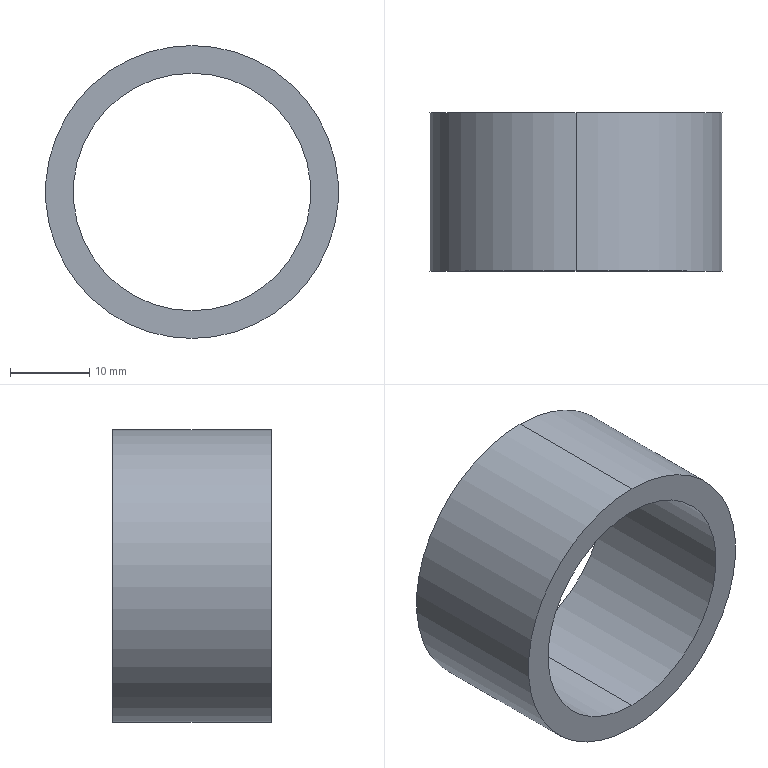Part | SolidWorks | features BaseBody 1 | 1 solid | 6 faces | box 37 x 20 x 37 mm | volume 7367 mm3 | cylinder 4 | plane 2 | commonest cylinder face diameters 30 x2 37 x2
STEP:
#1=CARTESIAN_POINT('',(-1069.592,-42.18,74.5));
#2=VERTEX_POINT('',#1);
#3=CARTESIAN_POINT('',(-1069.592,-22.18,74.5));
#4=VERTEX_POINT('',#3);
#5=CARTESIAN_POINT('',(-1069.592,-42.18,74.5));
#6=DIRECTION('',(0.,1.,0.));
#7=VECTOR('',#6,1000.);
#8=LINE('',#5,#7);
#9=EDGE_CURVE('',#2,#4,#8,.T.);
#10=ORIENTED_EDGE('',*,*,#9,.F.);
#11=CARTESIAN_POINT('',(-1069.592,-42.18,104.5));
#12=VERTEX_POINT('',#11);
#13=CARTESIAN_POINT('',(-1069.592,-42.18,89.5));
#14=DIRECTION('',(0.,1.,0.));
#15=DIRECTION('',(0.,0.,1.));
#16=AXIS2_PLACEMENT_3D('',#13,#14,#15);
#17=CIRCLE('',#16,15.);
#18=EDGE_CURVE('',#12,#2,#17,.T.);
#19=ORIENTED_EDGE('',*,*,#18,.F.);
#20=CARTESIAN_POINT('',(-1069.592,-22.18,104.5));
#21=VERTEX_POINT('',#20);
#22=CARTESIAN_POINT('',(-1069.592,-42.18,104.5));
#23=DIRECTION('',(0.,1.,0.));
#24=VECTOR('',#23,1000.);
#25=LINE('',#22,#24);
#26=EDGE_CURVE('',#12,#21,#25,.T.);
#27=ORIENTED_EDGE('',*,*,#26,.T.);
#28=CARTESIAN_POINT('',(-1069.592,-22.18,89.5));
#29=DIRECTION('',(0.,1.,0.));
#30=DIRECTION('',(0.,0.,1.));
#31=AXIS2_PLACEMENT_3D('',#28,#29,#30);
#32=CIRCLE('',#31,15.);
#33=EDGE_CURVE('',#21,#4,#32,.T.);
#34=ORIENTED_EDGE('',*,*,#33,.T.);
#35=EDGE_LOOP('',(#10,#19,#27,#34));
#36=FACE_OUTER_BOUND('',#35,.T.);
#37=CARTESIAN_POINT('',(-1069.592,-42.18,89.5));
#38=DIRECTION('',(0.,1.,0.));
#39=DIRECTION('',(0.,0.,1.));
#40=AXIS2_PLACEMENT_3D('',#37,#38,#39);
#41=CYLINDRICAL_SURFACE('',#40,15.);
#42=ADVANCED_FACE('',(#36),#41,.F.);
#43=CARTESIAN_POINT('',(-1069.592,-42.18,108.));
#44=VERTEX_POINT('',#43);
#45=CARTESIAN_POINT('',(-1069.592,-42.18,71.));
#46=VERTEX_POINT('',#45);
#47=CARTESIAN_POINT('',(-1069.592,-42.18,89.5));
#48=DIRECTION('',(0.,1.,0.));
#49=DIRECTION('',(0.,0.,1.));
#50=AXIS2_PLACEMENT_3D('',#47,#48,#49);
#51=CIRCLE('',#50,18.5);
#52=EDGE_CURVE('',#44,#46,#51,.T.);
#53=ORIENTED_EDGE('',*,*,#52,.F.);
#54=CARTESIAN_POINT('',(-1069.592,-42.18,89.5));
#55=DIRECTION('',(0.,1.,0.));
#56=DIRECTION('',(0.,0.,1.));
#57=AXIS2_PLACEMENT_3D('',#54,#55,#56);
#58=CIRCLE('',#57,18.5);
#59=EDGE_CURVE('',#46,#44,#58,.T.);
#60=ORIENTED_EDGE('',*,*,#59,.F.);
#61=EDGE_LOOP('',(#53,#60));
#62=FACE_OUTER_BOUND('',#61,.T.);
#63=ORIENTED_EDGE('',*,*,#18,.T.);
#64=CARTESIAN_POINT('',(-1069.592,-42.18,89.5));
#65=DIRECTION('',(0.,1.,0.));
#66=DIRECTION('',(0.,0.,1.));
#67=AXIS2_PLACEMENT_3D('',#64,#65,#66);
#68=CIRCLE('',#67,15.);
#69=EDGE_CURVE('',#2,#12,#68,.T.);
#70=ORIENTED_EDGE('',*,*,#69,.T.);
#71=EDGE_LOOP('',(#63,#70));
#72=FACE_BOUND('',#71,.T.);
#73=CARTESIAN_POINT('',(-1069.592,-42.18,89.5));
#74=DIRECTION('',(0.,-1.,0.));
#75=DIRECTION('',(-1.,0.,0.));
#76=AXIS2_PLACEMENT_3D('',#73,#74,#75);
#77=PLANE('',#76);
#78=ADVANCED_FACE('',(#62,#72),#77,.T.);
#79=CARTESIAN_POINT('',(-1069.592,-22.18,108.));
#80=VERTEX_POINT('',#79);
#81=CARTESIAN_POINT('',(-1069.592,-22.18,71.));
#82=VERTEX_POINT('',#81);
#83=CARTESIAN_POINT('',(-1069.592,-22.18,89.5));
#84=DIRECTION('',(0.,-1.,0.));
#85=DIRECTION('',(0.,0.,1.));
#86=AXIS2_PLACEMENT_3D('',#83,#84,#85);
#87=CIRCLE('',#86,18.5);
#88=EDGE_CURVE('',#80,#82,#87,.T.);
#89=ORIENTED_EDGE('',*,*,#88,.F.);
#90=CARTESIAN_POINT('',(-1069.592,-22.18,89.5));
#91=DIRECTION('',(0.,-1.,0.));
#92=DIRECTION('',(0.,0.,1.));
#93=AXIS2_PLACEMENT_3D('',#90,#91,#92);
#94=CIRCLE('',#93,18.5);
#95=EDGE_CURVE('',#82,#80,#94,.T.);
#96=ORIENTED_EDGE('',*,*,#95,.F.);
#97=EDGE_LOOP('',(#89,#96));
#98=FACE_OUTER_BOUND('',#97,.T.);
#99=ORIENTED_EDGE('',*,*,#33,.F.);
#100=CARTESIAN_POINT('',(-1069.592,-22.18,89.5));
#101=DIRECTION('',(0.,1.,0.));
#102=DIRECTION('',(0.,0.,1.));
#103=AXIS2_PLACEMENT_3D('',#100,#101,#102);
#104=CIRCLE('',#103,15.);
#105=EDGE_CURVE('',#4,#21,#104,.T.);
#106=ORIENTED_EDGE('',*,*,#105,.F.);
#107=EDGE_LOOP('',(#99,#106));
#108=FACE_BOUND('',#107,.T.);
#109=CARTESIAN_POINT('',(-1069.592,-22.18,89.5));
#110=DIRECTION('',(0.,-1.,0.));
#111=DIRECTION('',(-1.,0.,0.));
#112=AXIS2_PLACEMENT_3D('',#109,#110,#111);
#113=PLANE('',#112);
#114=ADVANCED_FACE('',(#98,#108),#113,.F.);
#115=CARTESIAN_POINT('',(-1069.592,-42.18,71.));
#116=DIRECTION('',(0.,1.,0.));
#117=VECTOR('',#116,1000.);
#118=LINE('',#115,#117);
#119=EDGE_CURVE('',#46,#82,#118,.T.);
#120=ORIENTED_EDGE('',*,*,#119,.F.);
#121=ORIENTED_EDGE('',*,*,#59,.T.);
#122=CARTESIAN_POINT('',(-1069.592,-42.18,108.));
#123=DIRECTION('',(0.,1.,0.));
#124=VECTOR('',#123,1000.);
#125=LINE('',#122,#124);
#126=EDGE_CURVE('',#44,#80,#125,.T.);
#127=ORIENTED_EDGE('',*,*,#126,.T.);
#128=ORIENTED_EDGE('',*,*,#88,.T.);
#129=EDGE_LOOP('',(#120,#121,#127,#128));
#130=FACE_OUTER_BOUND('',#129,.T.);
#131=CARTESIAN_POINT('',(-1069.592,-42.18,89.5));
#132=DIRECTION('',(0.,1.,0.));
#133=DIRECTION('',(0.,0.,1.));
#134=AXIS2_PLACEMENT_3D('',#131,#132,#133);
#135=CYLINDRICAL_SURFACE('',#134,18.5);
#136=ADVANCED_FACE('',(#130),#135,.T.);
#137=ORIENTED_EDGE('',*,*,#69,.F.);
#138=ORIENTED_EDGE('',*,*,#9,.T.);
#139=ORIENTED_EDGE('',*,*,#105,.T.);
#140=ORIENTED_EDGE('',*,*,#26,.F.);
#141=EDGE_LOOP('',(#137,#138,#139,#140));
#142=FACE_OUTER_BOUND('',#141,.T.);
#143=CARTESIAN_POINT('',(-1069.592,-42.18,89.5));
#144=DIRECTION('',(0.,1.,0.));
#145=DIRECTION('',(0.,0.,1.));
#146=AXIS2_PLACEMENT_3D('',#143,#144,#145);
#147=CYLINDRICAL_SURFACE('',#146,15.);
#148=ADVANCED_FACE('',(#142),#147,.F.);
#149=ORIENTED_EDGE('',*,*,#52,.T.);
#150=ORIENTED_EDGE('',*,*,#119,.T.);
#151=ORIENTED_EDGE('',*,*,#95,.T.);
#152=ORIENTED_EDGE('',*,*,#126,.F.);
#153=EDGE_LOOP('',(#149,#150,#151,#152));
#154=FACE_OUTER_BOUND('',#153,.T.);
#155=CARTESIAN_POINT('',(-1069.592,-42.18,89.5));
#156=DIRECTION('',(0.,1.,0.));
#157=DIRECTION('',(0.,0.,1.));
#158=AXIS2_PLACEMENT_3D('',#155,#156,#157);
#159=CYLINDRICAL_SURFACE('',#158,18.5);
#160=ADVANCED_FACE('',(#154),#159,.T.);
#161=CLOSED_SHELL('',(#42,#78,#114,#136,#148,#160));
#162=MANIFOLD_SOLID_BREP('',#161);
#163=CARTESIAN_POINT('',(0.,0.,0.));
#164=DIRECTION('',(0.,0.,1.));
#165=DIRECTION('',(1.,0.,0.));
#166=AXIS2_PLACEMENT_3D('',#163,#164,#165);
#167=(LENGTH_UNIT()NAMED_UNIT(*)SI_UNIT(.MILLI.,.METRE.));
#168=UNCERTAINTY_MEASURE_WITH_UNIT(LENGTH_MEASURE(0.00001),#167,'','');
#169=(NAMED_UNIT(*)PLANE_ANGLE_UNIT()SI_UNIT($,.RADIAN.));
#170=(NAMED_UNIT(*)SI_UNIT($,.STERADIAN.)SOLID_ANGLE_UNIT());
#171=(GEOMETRIC_REPRESENTATION_CONTEXT(3)GLOBAL_UNCERTAINTY_ASSIGNED_CONTEXT((#168))GLOBAL_UNIT_ASSIGNED_CONTEXT((#167,#169,#170))REPRESENTATION_CONTEXT('',''));
#172=ADVANCED_BREP_SHAPE_REPRESENTATION('',(#162,#166),#171);